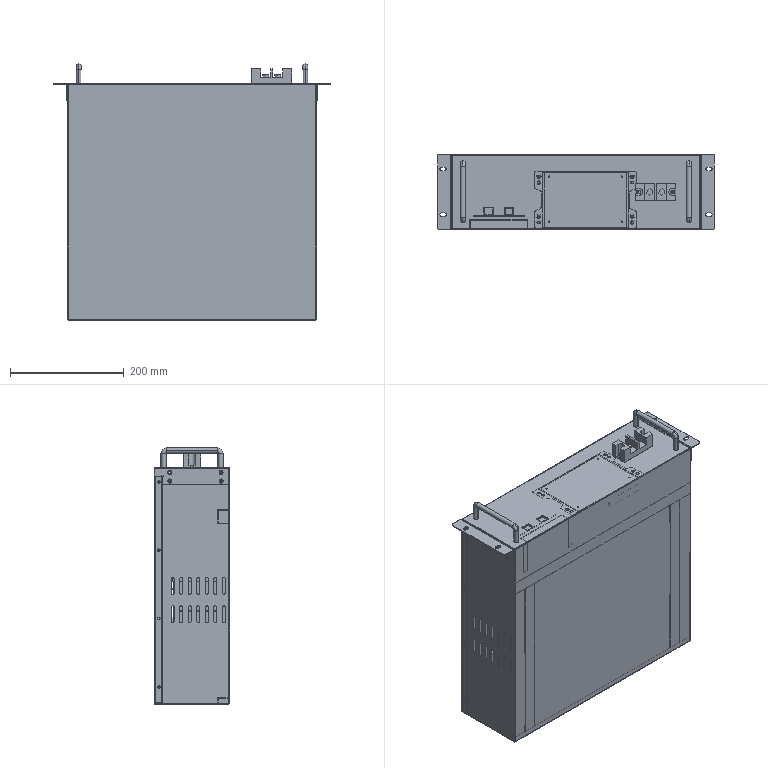Part | SolidWorks | features ReferencePattern 16, CompositeCurve 5, LocalLPattern 2, MirrorCompFeat 1 | 51 solids | 4391 faces | volume 10284410 mm3 | cylinder 2204 | plane 2093 | cone 46 | spline 38 | torus 8 | sphere 2 | commonest cylinder face diameters 0.305 x890 5 x128 0.889 x112 1 x111 12 x66 0.6 x64